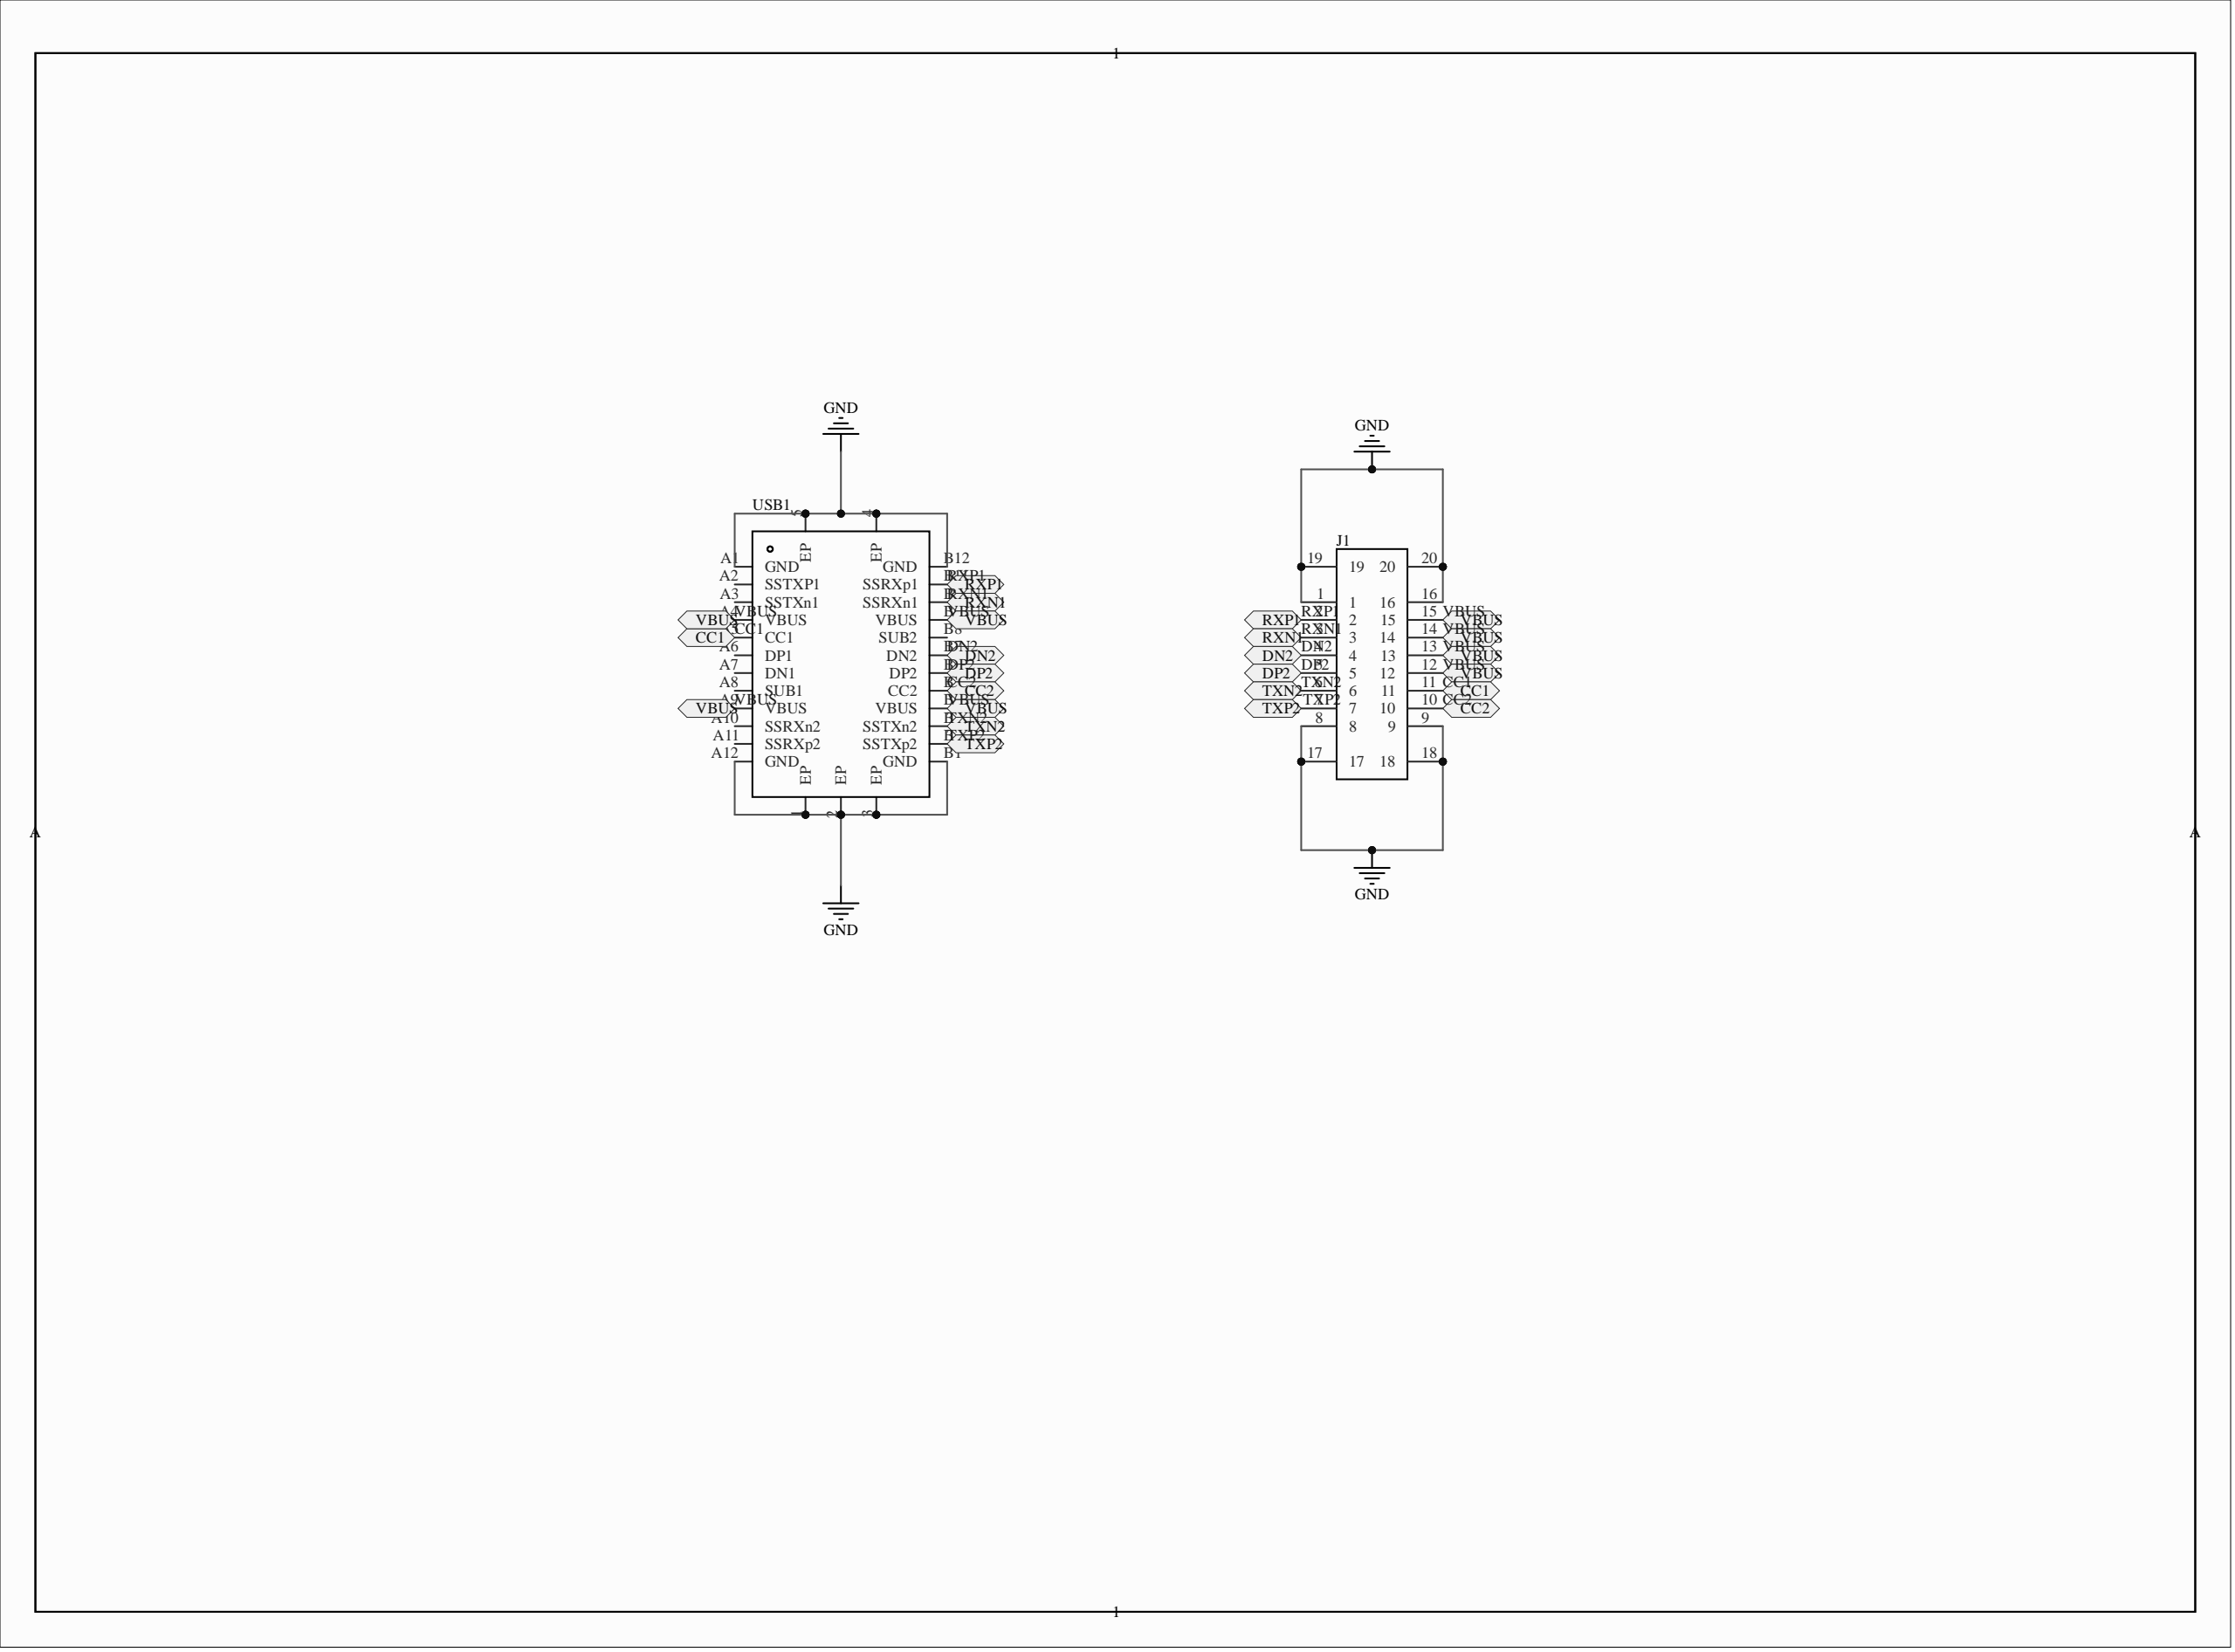Circuit board | Altium Designer | 2 parts | 10 nets
Bill of materials:
Comment,Description,Designator,Footprint,LibRef,Quantity
"BK13C06-16DS","2-0.35V(800)","J1","BK13C06-16DS_AA","BK13C06-16DS","1"
"TYPEC-952-ACP24","","USB1","USB-C-SMD_TYPEC-952-ACP24","TYPEC-952-ACP24","1"
Netlist (Protel format):
[
J1
BK13C06-16DS_AA
BK13C06-16DS



]
[
USB1
USB-C-SMD_TYPEC-952-ACP24
TYPEC-952-ACP24



]
(
VBUS
J1-12
J1-13
J1-14
J1-15
USB1-A4
USB1-A9
USB1-B4
USB1-B9
)
(
TXP2
J1-7
USB1-B2
)
(
TXN2
J1-6
USB1-B3
)
(
RXP1
J1-2
USB1-B11
)
(
RXN1
J1-3
USB1-B10
)
(
GND
J1-1
J1-8
J1-9
J1-16
J1-17
J1-18
J1-19
J1-20
USB1-1
USB1-2
USB1-3
USB1-4
USB1-5
USB1-A1
USB1-A12
USB1-B1
USB1-B12
)
(
DP2
J1-5
USB1-B6
)
(
DN2
J1-4
USB1-B7
)
(
CC2
J1-10
USB1-B5
)
(
CC1
J1-11
USB1-A5
)